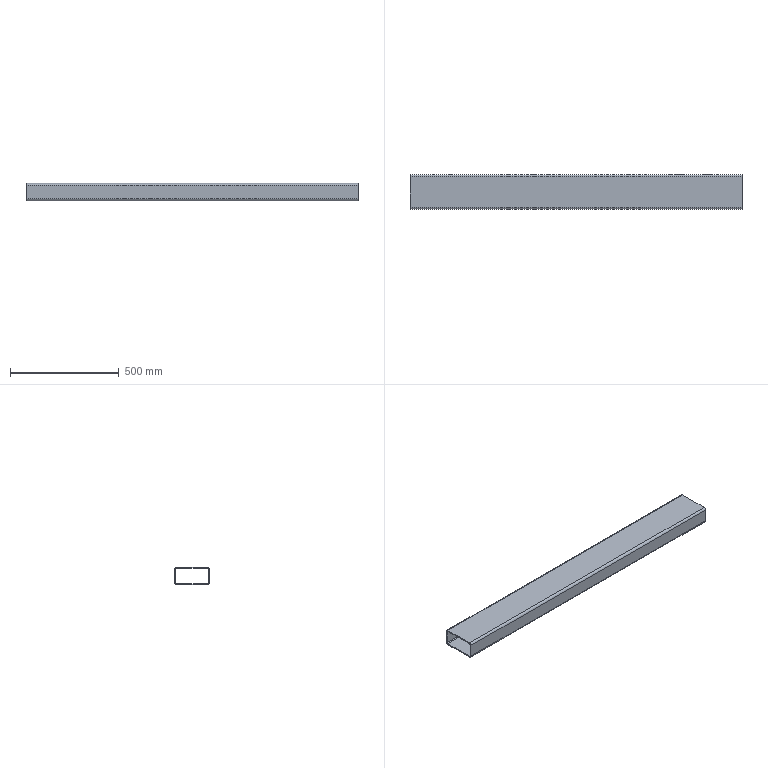Part | SolidWorks | features BaseBody 1 | 1 solid | 42 faces | box 1530 x 160 x 80 mm | volume 3404780 mm3 | cylinder 32 | plane 10 | commonest cylinder face diameters 8.5 x20 10 x4 20 x4 40.497 x4
STEP:
#1=CARTESIAN_POINT('',(324.25,75.,0.));
#2=VERTEX_POINT('',#1);
#3=CARTESIAN_POINT('',(315.75,75.,0.));
#4=VERTEX_POINT('',#3);
#5=CARTESIAN_POINT('',(320.,75.,0.));
#6=DIRECTION('',(0.,-1.,0.));
#7=DIRECTION('',(0.,0.,-1.));
#8=AXIS2_PLACEMENT_3D('',#5,#6,#7);
#9=CIRCLE('',#8,4.25);
#10=EDGE_CURVE('',#2,#4,#9,.T.);
#11=ORIENTED_EDGE('',*,*,#10,.T.);
#12=CARTESIAN_POINT('',(315.75,80.,0.));
#13=VERTEX_POINT('',#12);
#14=CARTESIAN_POINT('',(315.75,90.,0.));
#15=DIRECTION('',(0.,1.,0.));
#16=VECTOR('',#15,1000.);
#17=LINE('',#14,#16);
#18=EDGE_CURVE('',#4,#13,#17,.T.);
#19=ORIENTED_EDGE('',*,*,#18,.T.);
#20=CARTESIAN_POINT('',(324.25,80.,0.));
#21=VERTEX_POINT('',#20);
#22=CARTESIAN_POINT('',(320.,80.,0.));
#23=DIRECTION('',(0.,-1.,0.));
#24=DIRECTION('',(0.,0.,-1.));
#25=AXIS2_PLACEMENT_3D('',#22,#23,#24);
#26=CIRCLE('',#25,4.25);
#27=EDGE_CURVE('',#21,#13,#26,.T.);
#28=ORIENTED_EDGE('',*,*,#27,.F.);
#29=CARTESIAN_POINT('',(324.25,90.,0.));
#30=DIRECTION('',(0.,1.,0.));
#31=VECTOR('',#30,1000.);
#32=LINE('',#29,#31);
#33=EDGE_CURVE('',#2,#21,#32,.T.);
#34=ORIENTED_EDGE('',*,*,#33,.F.);
#35=EDGE_LOOP('',(#11,#19,#28,#34));
#36=FACE_OUTER_BOUND('',#35,.T.);
#37=CARTESIAN_POINT('',(320.,90.,0.));
#38=DIRECTION('',(0.,1.,0.));
#39=DIRECTION('',(1.,0.,0.));
#40=AXIS2_PLACEMENT_3D('',#37,#38,#39);
#41=CYLINDRICAL_SURFACE('',#40,4.25);
#42=ADVANCED_FACE('',(#36),#41,.F.);
#43=CARTESIAN_POINT('',(244.25,75.,0.));
#44=VERTEX_POINT('',#43);
#45=CARTESIAN_POINT('',(235.75,75.,0.));
#46=VERTEX_POINT('',#45);
#47=CARTESIAN_POINT('',(240.,75.,0.));
#48=DIRECTION('',(0.,-1.,0.));
#49=DIRECTION('',(0.,0.,-1.));
#50=AXIS2_PLACEMENT_3D('',#47,#48,#49);
#51=CIRCLE('',#50,4.25);
#52=EDGE_CURVE('',#44,#46,#51,.T.);
#53=ORIENTED_EDGE('',*,*,#52,.T.);
#54=CARTESIAN_POINT('',(235.75,80.,0.));
#55=VERTEX_POINT('',#54);
#56=CARTESIAN_POINT('',(235.75,90.,0.));
#57=DIRECTION('',(0.,1.,0.));
#58=VECTOR('',#57,1000.);
#59=LINE('',#56,#58);
#60=EDGE_CURVE('',#46,#55,#59,.T.);
#61=ORIENTED_EDGE('',*,*,#60,.T.);
#62=CARTESIAN_POINT('',(244.25,80.,0.));
#63=VERTEX_POINT('',#62);
#64=CARTESIAN_POINT('',(240.,80.,0.));
#65=DIRECTION('',(0.,-1.,0.));
#66=DIRECTION('',(0.,0.,-1.));
#67=AXIS2_PLACEMENT_3D('',#64,#65,#66);
#68=CIRCLE('',#67,4.25);
#69=EDGE_CURVE('',#63,#55,#68,.T.);
#70=ORIENTED_EDGE('',*,*,#69,.F.);
#71=CARTESIAN_POINT('',(244.25,90.,0.));
#72=DIRECTION('',(0.,1.,0.));
#73=VECTOR('',#72,1000.);
#74=LINE('',#71,#73);
#75=EDGE_CURVE('',#44,#63,#74,.T.);
#76=ORIENTED_EDGE('',*,*,#75,.F.);
#77=EDGE_LOOP('',(#53,#61,#70,#76));
#78=FACE_OUTER_BOUND('',#77,.T.);
#79=CARTESIAN_POINT('',(240.,90.,0.));
#80=DIRECTION('',(0.,1.,0.));
#81=DIRECTION('',(1.,0.,0.));
#82=AXIS2_PLACEMENT_3D('',#79,#80,#81);
#83=CYLINDRICAL_SURFACE('',#82,4.25);
#84=ADVANCED_FACE('',(#78),#83,.F.);
#85=CARTESIAN_POINT('',(-125.75,75.,0.));
#86=VERTEX_POINT('',#85);
#87=CARTESIAN_POINT('',(-134.25,75.,0.));
#88=VERTEX_POINT('',#87);
#89=CARTESIAN_POINT('',(-130.,75.,0.));
#90=DIRECTION('',(0.,-1.,0.));
#91=DIRECTION('',(0.,0.,-1.));
#92=AXIS2_PLACEMENT_3D('',#89,#90,#91);
#93=CIRCLE('',#92,4.25);
#94=EDGE_CURVE('',#86,#88,#93,.T.);
#95=ORIENTED_EDGE('',*,*,#94,.T.);
#96=CARTESIAN_POINT('',(-134.25,80.,0.));
#97=VERTEX_POINT('',#96);
#98=CARTESIAN_POINT('',(-134.25,90.,0.));
#99=DIRECTION('',(0.,1.,0.));
#100=VECTOR('',#99,1000.);
#101=LINE('',#98,#100);
#102=EDGE_CURVE('',#88,#97,#101,.T.);
#103=ORIENTED_EDGE('',*,*,#102,.T.);
#104=CARTESIAN_POINT('',(-125.75,80.,0.));
#105=VERTEX_POINT('',#104);
#106=CARTESIAN_POINT('',(-130.,80.,0.));
#107=DIRECTION('',(0.,-1.,0.));
#108=DIRECTION('',(0.,0.,-1.));
#109=AXIS2_PLACEMENT_3D('',#106,#107,#108);
#110=CIRCLE('',#109,4.25);
#111=EDGE_CURVE('',#105,#97,#110,.T.);
#112=ORIENTED_EDGE('',*,*,#111,.F.);
#113=CARTESIAN_POINT('',(-125.75,90.,0.));
#114=DIRECTION('',(0.,1.,0.));
#115=VECTOR('',#114,1000.);
#116=LINE('',#113,#115);
#117=EDGE_CURVE('',#86,#105,#116,.T.);
#118=ORIENTED_EDGE('',*,*,#117,.F.);
#119=EDGE_LOOP('',(#95,#103,#112,#118));
#120=FACE_OUTER_BOUND('',#119,.T.);
#121=CARTESIAN_POINT('',(-130.,90.,0.));
#122=DIRECTION('',(0.,1.,0.));
#123=DIRECTION('',(1.,0.,0.));
#124=AXIS2_PLACEMENT_3D('',#121,#122,#123);
#125=CYLINDRICAL_SURFACE('',#124,4.25);
#126=ADVANCED_FACE('',(#120),#125,.F.);
#127=CARTESIAN_POINT('',(-205.75,75.,0.));
#128=VERTEX_POINT('',#127);
#129=CARTESIAN_POINT('',(-214.25,75.,0.));
#130=VERTEX_POINT('',#129);
#131=CARTESIAN_POINT('',(-210.,75.,0.));
#132=DIRECTION('',(0.,-1.,0.));
#133=DIRECTION('',(0.,0.,-1.));
#134=AXIS2_PLACEMENT_3D('',#131,#132,#133);
#135=CIRCLE('',#134,4.25);
#136=EDGE_CURVE('',#128,#130,#135,.T.);
#137=ORIENTED_EDGE('',*,*,#136,.T.);
#138=CARTESIAN_POINT('',(-214.25,80.,0.));
#139=VERTEX_POINT('',#138);
#140=CARTESIAN_POINT('',(-214.25,90.,0.));
#141=DIRECTION('',(0.,1.,0.));
#142=VECTOR('',#141,1000.);
#143=LINE('',#140,#142);
#144=EDGE_CURVE('',#130,#139,#143,.T.);
#145=ORIENTED_EDGE('',*,*,#144,.T.);
#146=CARTESIAN_POINT('',(-205.75,80.,0.));
#147=VERTEX_POINT('',#146);
#148=CARTESIAN_POINT('',(-210.,80.,0.));
#149=DIRECTION('',(0.,-1.,0.));
#150=DIRECTION('',(0.,0.,-1.));
#151=AXIS2_PLACEMENT_3D('',#148,#149,#150);
#152=CIRCLE('',#151,4.25);
#153=EDGE_CURVE('',#147,#139,#152,.T.);
#154=ORIENTED_EDGE('',*,*,#153,.F.);
#155=CARTESIAN_POINT('',(-205.75,90.,0.));
#156=DIRECTION('',(0.,1.,0.));
#157=VECTOR('',#156,1000.);
#158=LINE('',#155,#157);
#159=EDGE_CURVE('',#128,#147,#158,.T.);
#160=ORIENTED_EDGE('',*,*,#159,.F.);
#161=EDGE_LOOP('',(#137,#145,#154,#160));
#162=FACE_OUTER_BOUND('',#161,.T.);
#163=CARTESIAN_POINT('',(-210.,90.,0.));
#164=DIRECTION('',(0.,1.,0.));
#165=DIRECTION('',(1.,0.,0.));
#166=AXIS2_PLACEMENT_3D('',#163,#164,#165);
#167=CYLINDRICAL_SURFACE('',#166,4.25);
#168=ADVANCED_FACE('',(#162),#167,.F.);
#169=CARTESIAN_POINT('',(-575.75,75.,0.));
#170=VERTEX_POINT('',#169);
#171=CARTESIAN_POINT('',(-584.25,75.,0.));
#172=VERTEX_POINT('',#171);
#173=CARTESIAN_POINT('',(-580.,75.,0.));
#174=DIRECTION('',(0.,-1.,0.));
#175=DIRECTION('',(0.,0.,-1.));
#176=AXIS2_PLACEMENT_3D('',#173,#174,#175);
#177=CIRCLE('',#176,4.25);
#178=EDGE_CURVE('',#170,#172,#177,.T.);
#179=ORIENTED_EDGE('',*,*,#178,.T.);
#180=CARTESIAN_POINT('',(-584.25,80.,0.));
#181=VERTEX_POINT('',#180);
#182=CARTESIAN_POINT('',(-584.25,90.,0.));
#183=DIRECTION('',(0.,1.,0.));
#184=VECTOR('',#183,1000.);
#185=LINE('',#182,#184);
#186=EDGE_CURVE('',#172,#181,#185,.T.);
#187=ORIENTED_EDGE('',*,*,#186,.T.);
#188=CARTESIAN_POINT('',(-575.75,80.,0.));
#189=VERTEX_POINT('',#188);
#190=CARTESIAN_POINT('',(-580.,80.,0.));
#191=DIRECTION('',(0.,-1.,0.));
#192=DIRECTION('',(0.,0.,-1.));
#193=AXIS2_PLACEMENT_3D('',#190,#191,#192);
#194=CIRCLE('',#193,4.25);
#195=EDGE_CURVE('',#189,#181,#194,.T.);
#196=ORIENTED_EDGE('',*,*,#195,.F.);
#197=CARTESIAN_POINT('',(-575.75,90.,0.));
#198=DIRECTION('',(0.,1.,0.));
#199=VECTOR('',#198,1000.);
#200=LINE('',#197,#199);
#201=EDGE_CURVE('',#170,#189,#200,.T.);
#202=ORIENTED_EDGE('',*,*,#201,.F.);
#203=EDGE_LOOP('',(#179,#187,#196,#202));
#204=FACE_OUTER_BOUND('',#203,.T.);
#205=CARTESIAN_POINT('',(-580.,90.,0.));
#206=DIRECTION('',(0.,1.,0.));
#207=DIRECTION('',(1.,0.,0.));
#208=AXIS2_PLACEMENT_3D('',#205,#206,#207);
#209=CYLINDRICAL_SURFACE('',#208,4.25);
#210=ADVANCED_FACE('',(#204),#209,.F.);
#211=CARTESIAN_POINT('',(-655.75,75.,0.));
#212=VERTEX_POINT('',#211);
#213=CARTESIAN_POINT('',(-664.25,75.,0.));
#214=VERTEX_POINT('',#213);
#215=CARTESIAN_POINT('',(-660.,75.,0.));
#216=DIRECTION('',(0.,-1.,0.));
#217=DIRECTION('',(0.,0.,-1.));
#218=AXIS2_PLACEMENT_3D('',#215,#216,#217);
#219=CIRCLE('',#218,4.25);
#220=EDGE_CURVE('',#212,#214,#219,.T.);
#221=ORIENTED_EDGE('',*,*,#220,.T.);
#222=CARTESIAN_POINT('',(-664.25,80.,0.));
#223=VERTEX_POINT('',#222);
#224=CARTESIAN_POINT('',(-664.25,90.,0.));
#225=DIRECTION('',(0.,1.,0.));
#226=VECTOR('',#225,1000.);
#227=LINE('',#224,#226);
#228=EDGE_CURVE('',#214,#223,#227,.T.);
#229=ORIENTED_EDGE('',*,*,#228,.T.);
#230=CARTESIAN_POINT('',(-655.75,80.,0.));
#231=VERTEX_POINT('',#230);
#232=CARTESIAN_POINT('',(-660.,80.,0.));
#233=DIRECTION('',(0.,-1.,0.));
#234=DIRECTION('',(0.,0.,-1.));
#235=AXIS2_PLACEMENT_3D('',#232,#233,#234);
#236=CIRCLE('',#235,4.25);
#237=EDGE_CURVE('',#231,#223,#236,.T.);
#238=ORIENTED_EDGE('',*,*,#237,.F.);
#239=CARTESIAN_POINT('',(-655.75,90.,0.));
#240=DIRECTION('',(0.,1.,0.));
#241=VECTOR('',#240,1000.);
#242=LINE('',#239,#241);
#243=EDGE_CURVE('',#212,#231,#242,.T.);
#244=ORIENTED_EDGE('',*,*,#243,.F.);
#245=EDGE_LOOP('',(#221,#229,#238,#244));
#246=FACE_OUTER_BOUND('',#245,.T.);
#247=CARTESIAN_POINT('',(-660.,90.,0.));
#248=DIRECTION('',(0.,1.,0.));
#249=DIRECTION('',(1.,0.,0.));
#250=AXIS2_PLACEMENT_3D('',#247,#248,#249);
#251=CYLINDRICAL_SURFACE('',#250,4.25);
#252=ADVANCED_FACE('',(#246),#251,.F.);
#253=CARTESIAN_POINT('',(627.748,75.,0.));
#254=VERTEX_POINT('',#253);
#255=CARTESIAN_POINT('',(587.252,75.,0.));
#256=VERTEX_POINT('',#255);
#257=CARTESIAN_POINT('',(607.5,75.,0.));
#258=DIRECTION('',(0.,-1.,0.));
#259=DIRECTION('',(0.,0.,-1.));
#260=AXIS2_PLACEMENT_3D('',#257,#258,#259);
#261=CIRCLE('',#260,20.248);
#262=EDGE_CURVE('',#254,#256,#261,.T.);
#263=ORIENTED_EDGE('',*,*,#262,.T.);
#264=CARTESIAN_POINT('',(587.252,80.,0.));
#265=VERTEX_POINT('',#264);
#266=CARTESIAN_POINT('',(587.252,70.,0.));
#267=DIRECTION('',(0.,1.,0.));
#268=VECTOR('',#267,1000.);
#269=LINE('',#266,#268);
#270=EDGE_CURVE('',#256,#265,#269,.T.);
#271=ORIENTED_EDGE('',*,*,#270,.T.);
#272=CARTESIAN_POINT('',(627.748,80.,0.));
#273=VERTEX_POINT('',#272);
#274=CARTESIAN_POINT('',(607.5,80.,0.));
#275=DIRECTION('',(0.,-1.,0.));
#276=DIRECTION('',(0.,0.,-1.));
#277=AXIS2_PLACEMENT_3D('',#274,#275,#276);
#278=CIRCLE('',#277,20.248);
#279=EDGE_CURVE('',#273,#265,#278,.T.);
#280=ORIENTED_EDGE('',*,*,#279,.F.);
#281=CARTESIAN_POINT('',(627.748,70.,0.));
#282=DIRECTION('',(0.,1.,0.));
#283=VECTOR('',#282,1000.);
#284=LINE('',#281,#283);
#285=EDGE_CURVE('',#254,#273,#284,.T.);
#286=ORIENTED_EDGE('',*,*,#285,.F.);
#287=EDGE_LOOP('',(#263,#271,#280,#286));
#288=FACE_OUTER_BOUND('',#287,.T.);
#289=CARTESIAN_POINT('',(607.5,70.,0.));
#290=DIRECTION('',(0.,1.,0.));
#291=DIRECTION('',(1.,0.,0.));
#292=AXIS2_PLACEMENT_3D('',#289,#290,#291);
#293=CYLINDRICAL_SURFACE('',#292,20.248);
#294=ADVANCED_FACE('',(#288),#293,.F.);
#295=CARTESIAN_POINT('',(492.748,75.,0.));
#296=VERTEX_POINT('',#295);
#297=CARTESIAN_POINT('',(452.252,75.,0.));
#298=VERTEX_POINT('',#297);
#299=CARTESIAN_POINT('',(472.5,75.,0.));
#300=DIRECTION('',(0.,-1.,0.));
#301=DIRECTION('',(0.,0.,-1.));
#302=AXIS2_PLACEMENT_3D('',#299,#300,#301);
#303=CIRCLE('',#302,20.248);
#304=EDGE_CURVE('',#296,#298,#303,.T.);
#305=ORIENTED_EDGE('',*,*,#304,.T.);
#306=CARTESIAN_POINT('',(452.252,80.,0.));
#307=VERTEX_POINT('',#306);
#308=CARTESIAN_POINT('',(452.252,70.,0.));
#309=DIRECTION('',(0.,1.,0.));
#310=VECTOR('',#309,1000.);
#311=LINE('',#308,#310);
#312=EDGE_CURVE('',#298,#307,#311,.T.);
#313=ORIENTED_EDGE('',*,*,#312,.T.);
#314=CARTESIAN_POINT('',(492.748,80.,0.));
#315=VERTEX_POINT('',#314);
#316=CARTESIAN_POINT('',(472.5,80.,0.));
#317=DIRECTION('',(0.,-1.,0.));
#318=DIRECTION('',(0.,0.,-1.));
#319=AXIS2_PLACEMENT_3D('',#316,#317,#318);
#320=CIRCLE('',#319,20.248);
#321=EDGE_CURVE('',#315,#307,#320,.T.);
#322=ORIENTED_EDGE('',*,*,#321,.F.);
#323=CARTESIAN_POINT('',(492.748,70.,0.));
#324=DIRECTION('',(0.,1.,0.));
#325=VECTOR('',#324,1000.);
#326=LINE('',#323,#325);
#327=EDGE_CURVE('',#296,#315,#326,.T.);
#328=ORIENTED_EDGE('',*,*,#327,.F.);
#329=EDGE_LOOP('',(#305,#313,#322,#328));
#330=FACE_OUTER_BOUND('',#329,.T.);
#331=CARTESIAN_POINT('',(472.5,70.,0.));
#332=DIRECTION('',(0.,1.,0.));
#333=DIRECTION('',(1.,0.,0.));
#334=AXIS2_PLACEMENT_3D('',#331,#332,#333);
#335=CYLINDRICAL_SURFACE('',#334,20.248);
#336=ADVANCED_FACE('',(#330),#335,.F.);
#337=CARTESIAN_POINT('',(436.75,75.,-15.));
#338=VERTEX_POINT('',#337);
#339=CARTESIAN_POINT('',(428.25,75.,-15.));
#340=VERTEX_POINT('',#339);
#341=CARTESIAN_POINT('',(432.5,75.,-15.));
#342=DIRECTION('',(0.,-1.,0.));
#343=DIRECTION('',(0.,0.,-1.));
#344=AXIS2_PLACEMENT_3D('',#341,#342,#343);
#345=CIRCLE('',#344,4.25);
#346=EDGE_CURVE('',#338,#340,#345,.T.);
#347=ORIENTED_EDGE('',*,*,#346,.T.);
#348=CARTESIAN_POINT('',(428.25,80.,-15.));
#349=VERTEX_POINT('',#348);
#350=CARTESIAN_POINT('',(428.25,90.,-15.));
#351=DIRECTION('',(0.,1.,0.));
#352=VECTOR('',#351,1000.);
#353=LINE('',#350,#352);
#354=EDGE_CURVE('',#340,#349,#353,.T.);
#355=ORIENTED_EDGE('',*,*,#354,.T.);
#356=CARTESIAN_POINT('',(436.75,80.,-15.));
#357=VERTEX_POINT('',#356);
#358=CARTESIAN_POINT('',(432.5,80.,-15.));
#359=DIRECTION('',(0.,-1.,0.));
#360=DIRECTION('',(0.,0.,-1.));
#361=AXIS2_PLACEMENT_3D('',#358,#359,#360);
#362=CIRCLE('',#361,4.25);
#363=EDGE_CURVE('',#357,#349,#362,.T.);
#364=ORIENTED_EDGE('',*,*,#363,.F.);
#365=CARTESIAN_POINT('',(436.75,90.,-15.));
#366=DIRECTION('',(0.,1.,0.));
#367=VECTOR('',#366,1000.);
#368=LINE('',#365,#367);
#369=EDGE_CURVE('',#338,#357,#368,.T.);
#370=ORIENTED_EDGE('',*,*,#369,.F.);
#371=EDGE_LOOP('',(#347,#355,#364,#370));
#372=FACE_OUTER_BOUND('',#371,.T.);
#373=CARTESIAN_POINT('',(432.5,90.,-15.));
#374=DIRECTION('',(0.,1.,0.));
#375=DIRECTION('',(1.,0.,0.));
#376=AXIS2_PLACEMENT_3D('',#373,#374,#375);
#377=CYLINDRICAL_SURFACE('',#376,4.25);
#378=ADVANCED_FACE('',(#372),#377,.F.);
#379=CARTESIAN_POINT('',(436.75,75.,15.));
#380=VERTEX_POINT('',#379);
#381=CARTESIAN_POINT('',(428.25,75.,15.));
#382=VERTEX_POINT('',#381);
#383=CARTESIAN_POINT('',(432.5,75.,15.));
#384=DIRECTION('',(0.,-1.,0.));
#385=DIRECTION('',(0.,0.,-1.));
#386=AXIS2_PLACEMENT_3D('',#383,#384,#385);
#387=CIRCLE('',#386,4.25);
#388=EDGE_CURVE('',#380,#382,#387,.T.);
#389=ORIENTED_EDGE('',*,*,#388,.T.);
#390=CARTESIAN_POINT('',(428.25,80.,15.));
#391=VERTEX_POINT('',#390);
#392=CARTESIAN_POINT('',(428.25,90.,15.));
#393=DIRECTION('',(0.,1.,0.));
#394=VECTOR('',#393,1000.);
#395=LINE('',#392,#394);
#396=EDGE_CURVE('',#382,#391,#395,.T.);
#397=ORIENTED_EDGE('',*,*,#396,.T.);
#398=CARTESIAN_POINT('',(436.75,80.,15.));
#399=VERTEX_POINT('',#398);
#400=CARTESIAN_POINT('',(432.5,80.,15.));
#401=DIRECTION('',(0.,-1.,0.));
#402=DIRECTION('',(0.,0.,-1.));
#403=AXIS2_PLACEMENT_3D('',#400,#401,#402);
#404=CIRCLE('',#403,4.25);
#405=EDGE_CURVE('',#399,#391,#404,.T.);
#406=ORIENTED_EDGE('',*,*,#405,.F.);
#407=CARTESIAN_POINT('',(436.75,90.,15.));
#408=DIRECTION('',(0.,1.,0.));
#409=VECTOR('',#408,1000.);
#410=LINE('',#407,#409);
#411=EDGE_CURVE('',#380,#399,#410,.T.);
#412=ORIENTED_EDGE('',*,*,#411,.F.);
#413=EDGE_LOOP('',(#389,#397,#406,#412));
#414=FACE_OUTER_BOUND('',#413,.T.);
#415=CARTESIAN_POINT('',(432.5,90.,15.));
#416=DIRECTION('',(0.,1.,0.));
#417=DIRECTION('',(1.,0.,0.));
#418=AXIS2_PLACEMENT_3D('',#415,#416,#417);
#419=CYLINDRICAL_SURFACE('',#418,4.25);
#420=ADVANCED_FACE('',(#414),#419,.F.);
#421=CARTESIAN_POINT('',(651.75,75.,15.));
#422=VERTEX_POINT('',#421);
#423=CARTESIAN_POINT('',(643.25,75.,15.));
#424=VERTEX_POINT('',#423);
#425=CARTESIAN_POINT('',(647.5,75.,15.));
#426=DIRECTION('',(0.,-1.,0.));
#427=DIRECTION('',(0.,0.,-1.));
#428=AXIS2_PLACEMENT_3D('',#425,#426,#427);
#429=CIRCLE('',#428,4.25);
#430=EDGE_CURVE('',#422,#424,#429,.T.);
#431=ORIENTED_EDGE('',*,*,#430,.T.);
#432=CARTESIAN_POINT('',(643.25,80.,15.));
#433=VERTEX_POINT('',#432);
#434=CARTESIAN_POINT('',(643.25,90.,15.));
#435=DIRECTION('',(0.,1.,0.));
#436=VECTOR('',#435,1000.);
#437=LINE('',#434,#436);
#438=EDGE_CURVE('',#424,#433,#437,.T.);
#439=ORIENTED_EDGE('',*,*,#438,.T.);
#440=CARTESIAN_POINT('',(651.75,80.,15.));
#441=VERTEX_POINT('',#440);
#442=CARTESIAN_POINT('',(647.5,80.,15.));
#443=DIRECTION('',(0.,-1.,0.));
#444=DIRECTION('',(0.,0.,-1.));
#445=AXIS2_PLACEMENT_3D('',#442,#443,#444);
#446=CIRCLE('',#445,4.25);
#447=EDGE_CURVE('',#441,#433,#446,.T.);
#448=ORIENTED_EDGE('',*,*,#447,.F.);
#449=CARTESIAN_POINT('',(651.75,90.,15.));
#450=DIRECTION('',(0.,1.,0.));
#451=VECTOR('',#450,1000.);
#452=LINE('',#449,#451);
#453=EDGE_CURVE('',#422,#441,#452,.T.);
#454=ORIENTED_EDGE('',*,*,#453,.F.);
#455=EDGE_LOOP('',(#431,#439,#448,#454));
#456=FACE_OUTER_BOUND('',#455,.T.);
#457=CARTESIAN_POINT('',(647.5,90.,15.));
#458=DIRECTION('',(0.,1.,0.));
#459=DIRECTION('',(1.,0.,0.));
#460=AXIS2_PLACEMENT_3D('',#457,#458,#459);
#461=CYLINDRICAL_SURFACE('',#460,4.25);
#462=ADVANCED_FACE('',(#456),#461,.F.);
#463=CARTESIAN_POINT('',(651.75,75.,-15.));
#464=VERTEX_POINT('',#463);
#465=CARTESIAN_POINT('',(643.25,75.,-15.));
#466=VERTEX_POINT('',#465);
#467=CARTESIAN_POINT('',(647.5,75.,-15.));
#468=DIRECTION('',(0.,-1.,0.));
#469=DIRECTION('',(0.,0.,-1.));
#470=AXIS2_PLACEMENT_3D('',#467,#468,#469);
#471=CIRCLE('',#470,4.25);
#472=EDGE_CURVE('',#464,#466,#471,.T.);
#473=ORIENTED_EDGE('',*,*,#472,.T.);
#474=CARTESIAN_POINT('',(643.25,80.,-15.));
#475=VERTEX_POINT('',#474);
#476=CARTESIAN_POINT('',(643.25,90.,-15.));
#477=DIRECTION('',(0.,1.,0.));
#478=VECTOR('',#477,1000.);
#479=LINE('',#476,#478);
#480=EDGE_CURVE('',#466,#475,#479,.T.);
#481=ORIENTED_EDGE('',*,*,#480,.T.);
#482=CARTESIAN_POINT('',(651.75,80.,-15.));
#483=VERTEX_POINT('',#482);
#484=CARTESIAN_POINT('',(647.5,80.,-15.));
#485=DIRECTION('',(0.,-1.,0.));
#486=DIRECTION('',(0.,0.,-1.));
#487=AXIS2_PLACEMENT_3D('',#484,#485,#486);
#488=CIRCLE('',#487,4.25);
#489=EDGE_CURVE('',#483,#475,#488,.T.);
#490=ORIENTED_EDGE('',*,*,#489,.F.);
#491=CARTESIAN_POINT('',(651.75,90.,-15.));
#492=DIRECTION('',(0.,1.,0.));
#493=VECTOR('',#492,1000.);
#494=LINE('',#491,#493);
#495=EDGE_CURVE('',#464,#483,#494,.T.);
#496=ORIENTED_EDGE('',*,*,#495,.F.);
#497=EDGE_LOOP('',(#473,#481,#490,#496));
#498=FACE_OUTER_BOUND('',#497,.T.);
#499=CARTESIAN_POINT('',(647.5,90.,-15.));
#500=DIRECTION('',(0.,1.,0.));
#501=DIRECTION('',(1.,0.,0.));
#502=AXIS2_PLACEMENT_3D('',#499,#500,#501);
#503=CYLINDRICAL_SURFACE('',#502,4.25);
#504=ADVANCED_FACE('',(#498),#503,.F.);
#505=CARTESIAN_POINT('',(762.5,70.,-40.));
#506=VERTEX_POINT('',#505);
#507=CARTESIAN_POINT('',(762.5,80.,-30.));
#508=VERTEX_POINT('',#507);
#509=CARTESIAN_POINT('',(762.5,70.,-30.));
#510=DIRECTION('',(1.,0.,0.));
#511=DIRECTION('',(0.,1.,0.));
#512=AXIS2_PLACEMENT_3D('',#509,#510,#511);
#513=CIRCLE('',#512,10.);
#514=EDGE_CURVE('',#506,#508,#513,.T.);
#515=ORIENTED_EDGE('',*,*,#514,.F.);
#516=CARTESIAN_POINT('',(-767.5,70.,-40.));
#517=VERTEX_POINT('',#516);
#518=CARTESIAN_POINT('',(767.5,70.,-40.));
#519=DIRECTION('',(-1.,0.,0.));
#520=VECTOR('',#519,1000.);
#521=LINE('',#518,#520);
#522=EDGE_CURVE('',#506,#517,#521,.T.);
#523=ORIENTED_EDGE('',*,*,#522,.T.);
#524=CARTESIAN_POINT('',(-767.5,80.,-30.));
#525=VERTEX_POINT('',#524);
#526=CARTESIAN_POINT('',(-767.5,70.,-30.));
#527=DIRECTION('',(1.,0.,0.));
#528=DIRECTION('',(0.,0.,-1.));
#529=AXIS2_PLACEMENT_3D('',#526,#527,#528);
#530=CIRCLE('',#529,10.);
#531=EDGE_CURVE('',#517,#525,#530,.T.);
#532=ORIENTED_EDGE('',*,*,#531,.T.);
#533=CARTESIAN_POINT('',(767.5,80.,-30.));
#534=DIRECTION('',(-1.,0.,0.));
#535=VECTOR('',#534,1000.);
#536=LINE('',#533,#535);
#537=EDGE_CURVE('',#508,#525,#536,.T.);
#538=ORIENTED_EDGE('',*,*,#537,.F.);
#539=EDGE_LOOP('',(#515,#523,#532,#538));
#540=FACE_OUTER_BOUND('',#539,.T.);
#541=CARTESIAN_POINT('',(767.5,70.,-30.));
#542=DIRECTION('',(-1.,0.,0.));
#543=DIRECTION('',(0.,0.,1.));
#544=AXIS2_PLACEMENT_3D('',#541,#542,#543);
#545=CYLINDRICAL_SURFACE('',#544,10.);
#546=ADVANCED_FACE('',(#540),#545,.T.);
#547=ORIENTED_EDGE('',*,*,#27,.T.);
#548=CARTESIAN_POINT('',(320.,80.,0.));
#549=DIRECTION('',(0.,-1.,0.));
#550=DIRECTION('',(0.,0.,-1.));
#551=AXIS2_PLACEMENT_3D('',#548,#549,#550);
#552=CIRCLE('',#551,4.25);
#553=EDGE_CURVE('',#13,#21,#552,.T.);
#554=ORIENTED_EDGE('',*,*,#553,.T.);
#555=EDGE_LOOP('',(#547,#554));
#556=FACE_BOUND('',#555,.T.);
#557=ORIENTED_EDGE('',*,*,#69,.T.);
#558=CARTESIAN_POINT('',(240.,80.,0.));
#559=DIRECTION('',(0.,-1.,0.));
#560=DIRECTION('',(0.,0.,-1.));
#561=AXIS2_PLACEMENT_3D('',#558,#559,#560);
#562=CIRCLE('',#561,4.25);
#563=EDGE_CURVE('',#55,#63,#562,.T.);
#564=ORIENTED_EDGE('',*,*,#563,.T.);
#565=EDGE_LOOP('',(#557,#564));
#566=FACE_BOUND('',#565,.T.);
#567=ORIENTED_EDGE('',*,*,#111,.T.);
#568=CARTESIAN_POINT('',(-130.,80.,0.));
#569=DIRECTION('',(0.,-1.,0.));
#570=DIRECTION('',(0.,0.,-1.));
#571=AXIS2_PLACEMENT_3D('',#568,#569,#570);
#572=CIRCLE('',#571,4.25);
#573=EDGE_CURVE('',#97,#105,#572,.T.);
#574=ORIENTED_EDGE('',*,*,#573,.T.);
#575=EDGE_LOOP('',(#567,#574));
#576=FACE_BOUND('',#575,.T.);
#577=ORIENTED_EDGE('',*,*,#153,.T.);
#578=CARTESIAN_POINT('',(-210.,80.,0.));
#579=DIRECTION('',(0.,-1.,0.));
#580=DIRECTION('',(0.,0.,-1.));
#581=AXIS2_PLACEMENT_3D('',#578,#579,#580);
#582=CIRCLE('',#581,4.25);
#583=EDGE_CURVE('',#139,#147,#582,.T.);
#584=ORIENTED_EDGE('',*,*,#583,.T.);
#585=EDGE_LOOP('',(#577,#584));
#586=FACE_BOUND('',#585,.T.);
#587=ORIENTED_EDGE('',*,*,#195,.T.);
#588=CARTESIAN_POINT('',(-580.,80.,0.));
#589=DIRECTION('',(0.,-1.,0.));
#590=DIRECTION('',(0.,0.,-1.));
#591=AXIS2_PLACEMENT_3D('',#588,#589,#590);
#592=CIRCLE('',#591,4.25);
#593=EDGE_CURVE('',#181,#189,#592,.T.);
#594=ORIENTED_EDGE('',*,*,#593,.T.);
#595=EDGE_LOOP('',(#587,#594));
#596=FACE_BOUND('',#595,.T.);
#597=ORIENTED_EDGE('',*,*,#237,.T.);
#598=CARTESIAN_POINT('',(-660.,80.,0.));
#599=DIRECTION('',(0.,-1.,0.));
#600=DIRECTION('',(0.,0.,-1.));
#601=AXIS2_PLACEMENT_3D('',#598,#599,#600);
#602=CIRCLE('',#601,4.25);
#603=EDGE_CURVE('',#223,#231,#602,.T.);
#604=ORIENTED_EDGE('',*,*,#603,.T.);
#605=EDGE_LOOP('',(#597,#604));
#606=FACE_BOUND('',#605,.T.);
#607=ORIENTED_EDGE('',*,*,#279,.T.);
#608=CARTESIAN_POINT('',(607.5,80.,0.));
#609=DIRECTION('',(0.,-1.,0.));
#610=DIRECTION('',(0.,0.,-1.));
#611=AXIS2_PLACEMENT_3D('',#608,#609,#610);
#612=CIRCLE('',#611,20.248);
#613=EDGE_CURVE('',#265,#273,#612,.T.);
#614=ORIENTED_EDGE('',*,*,#613,.T.);
#615=EDGE_LOOP('',(#607,#614));
#616=FACE_BOUND('',#615,.T.);
#617=ORIENTED_EDGE('',*,*,#321,.T.);
#618=CARTESIAN_POINT('',(472.5,80.,0.));
#619=DIRECTION('',(0.,-1.,0.));
#620=DIRECTION('',(0.,0.,-1.));
#621=AXIS2_PLACEMENT_3D('',#618,#619,#620);
#622=CIRCLE('',#621,20.248);
#623=EDGE_CURVE('',#307,#315,#622,.T.);
#624=ORIENTED_EDGE('',*,*,#623,.T.);
#625=EDGE_LOOP('',(#617,#624));
#626=FACE_BOUND('',#625,.T.);
#627=ORIENTED_EDGE('',*,*,#363,.T.);
#628=CARTESIAN_POINT('',(432.5,80.,-15.));
#629=DIRECTION('',(0.,-1.,0.));
#630=DIRECTION('',(0.,0.,-1.));
#631=AXIS2_PLACEMENT_3D('',#628,#629,#630);
#632=CIRCLE('',#631,4.25);
#633=EDGE_CURVE('',#349,#357,#632,.T.);
#634=ORIENTED_EDGE('',*,*,#633,.T.);
#635=EDGE_LOOP('',(#627,#634));
#636=FACE_BOUND('',#635,.T.);
#637=ORIENTED_EDGE('',*,*,#405,.T.);
#638=CARTESIAN_POINT('',(432.5,80.,15.));
#639=DIRECTION('',(0.,-1.,0.));
#640=DIRECTION('',(0.,0.,-1.));
#641=AXIS2_PLACEMENT_3D('',#638,#639,#640);
#642=CIRCLE('',#641,4.25);
#643=EDGE_CURVE('',#391,#399,#642,.T.);
#644=ORIENTED_EDGE('',*,*,#643,.T.);
#645=EDGE_LOOP('',(#637,#644));
#646=FACE_BOUND('',#645,.T.);
#647=ORIENTED_EDGE('',*,*,#447,.T.);
#648=CARTESIAN_POINT('',(647.5,80.,15.));
#649=DIRECTION('',(0.,-1.,0.));
#650=DIRECTION('',(0.,0.,-1.));
#651=AXIS2_PLACEMENT_3D('',#648,#649,#650);
#652=CIRCLE('',#651,4.25);
#653=EDGE_CURVE('',#433,#441,#652,.T.);
#654=ORIENTED_EDGE('',*,*,#653,.T.);
#655=EDGE_LOOP('',(#647,#654));
#656=FACE_BOUND('',#655,.T.);
#657=ORIENTED_EDGE('',*,*,#489,.T.);
#658=CARTESIAN_POINT('',(647.5,80.,-15.));
#659=DIRECTION('',(0.,-1.,0.));
#660=DIRECTION('',(0.,0.,-1.));
#661=AXIS2_PLACEMENT_3D('',#658,#659,#660);
#662=CIRCLE('',#661,4.25);
#663=EDGE_CURVE('',#475,#483,#662,.T.);
#664=ORIENTED_EDGE('',*,*,#663,.T.);
#665=EDGE_LOOP('',(#657,#664));
#666=FACE_BOUND('',#665,.T.);
#667=CARTESIAN_POINT('',(762.5,80.,30.));
#668=VERTEX_POINT('',#667);
#669=CARTESIAN_POINT('',(762.5,80.,-30.));
#670=DIRECTION('',(0.,0.,1.));
#671=VECTOR('',#670,1000.);
#672=LINE('',#669,#671);
#673=EDGE_CURVE('',#508,#668,#672,.T.);
#674=ORIENTED_EDGE('',*,*,#673,.F.);
#675=ORIENTED_EDGE('',*,*,#537,.T.);
#676=CARTESIAN_POINT('',(-767.5,80.,30.));
#677=VERTEX_POINT('',#676);
#678=CARTESIAN_POINT('',(-767.5,80.,-30.));
#679=DIRECTION('',(0.,0.,1.));
#680=VECTOR('',#679,1000.);
#681=LINE('',#678,#680);
#682=EDGE_CURVE('',#525,#677,#681,.T.);
#683=ORIENTED_EDGE('',*,*,#682,.T.);
#684=CARTESIAN_POINT('',(767.5,80.,30.));
#685=DIRECTION('',(-1.,0.,0.));
#686=VECTOR('',#685,1000.);
#687=LINE('',#684,#686);
#688=EDGE_CURVE('',#668,#677,#687,.T.);
#689=ORIENTED_EDGE('',*,*,#688,.F.);
#690=EDGE_LOOP('',(#674,#675,#683,#689));
#691=FACE_OUTER_BOUND('',#690,.T.);
#692=CARTESIAN_POINT('',(767.5,80.,-30.));
#693=DIRECTION('',(0.,-1.,0.));
#694=DIRECTION('',(0.,0.,-1.));
#695=AXIS2_PLACEMENT_3D('',#692,#693,#694);
#696=PLANE('',#695);
#697=ADVANCED_FACE('',(#556,#566,#576,#586,#596,#606,#616,#626,#636,#646,#656,#666,#691),#696,.F.);
#698=CARTESIAN_POINT('',(762.5,70.,40.));
#699=VERTEX_POINT('',#698);
#700=CARTESIAN_POINT('',(762.5,70.,30.));
#701=DIRECTION('',(1.,0.,0.));
#702=DIRECTION('',(0.,1.,0.));
#703=AXIS2_PLACEMENT_3D('',#700,#701,#702);
#704=CIRCLE('',#703,10.);
#705=EDGE_CURVE('',#668,#699,#704,.T.);
#706=ORIENTED_EDGE('',*,*,#705,.F.);
#707=ORIENTED_EDGE('',*,*,#688,.T.);
#708=CARTESIAN_POINT('',(-767.5,70.,40.));
#709=VERTEX_POINT('',#708);
#710=CARTESIAN_POINT('',(-767.5,70.,30.));
#711=DIRECTION('',(1.,0.,0.));
#712=DIRECTION('',(0.,0.,-1.));
#713=AXIS2_PLACEMENT_3D('',#710,#711,#712);
#714=CIRCLE('',#713,10.);
#715=EDGE_CURVE('',#677,#709,#714,.T.);
#716=ORIENTED_EDGE('',*,*,#715,.T.);
#717=CARTESIAN_POINT('',(767.5,70.,40.));
#718=DIRECTION('',(-1.,0.,0.));
#719=VECTOR('',#718,1000.);
#720=LINE('',#717,#719);
#721=EDGE_CURVE('',#699,#709,#720,.T.);
#722=ORIENTED_EDGE('',*,*,#721,.F.);
#723=EDGE_LOOP('',(#706,#707,#716,#722));
#724=FACE_OUTER_BOUND('',#723,.T.);
#725=CARTESIAN_POINT('',(767.5,70.,30.));
#726=DIRECTION('',(-1.,0.,0.));
#727=DIRECTION('',(0.,0.,1.));
#728=AXIS2_PLACEMENT_3D('',#725,#726,#727);
#729=CYLINDRICAL_SURFACE('',#728,10.);
#730=ADVANCED_FACE('',(#724),#729,.T.);
#731=CARTESIAN_POINT('',(762.5,-70.,40.));
#732=VERTEX_POINT('',#731);
#733=CARTESIAN_POINT('',(762.5,-70.,40.));
#734=DIRECTION('',(0.,-1.,0.));
#735=VECTOR('',#734,1000.);
#736=LINE('',#733,#735);
#737=EDGE_CURVE('',#699,#732,#736,.T.);
#738=ORIENTED_EDGE('',*,*,#737,.F.);
#739=ORIENTED_EDGE('',*,*,#721,.T.);
#740=CARTESIAN_POINT('',(-767.5,-70.,40.));
#741=VERTEX_POINT('',#740);
#742=CARTESIAN_POINT('',(-767.5,-70.,40.));
#743=DIRECTION('',(0.,-1.,0.));
#744=VECTOR('',#743,1000.);
#745=LINE('',#742,#744);
#746=EDGE_CURVE('',#709,#741,#745,.T.);
#747=ORIENTED_EDGE('',*,*,#746,.T.);
#748=CARTESIAN_POINT('',(767.5,-70.,40.));
#749=DIRECTION('',(-1.,0.,0.));
#750=VECTOR('',#749,1000.);
#751=LINE('',#748,#750);
#752=EDGE_CURVE('',#732,#741,#751,.T.);
#753=ORIENTED_EDGE('',*,*,#752,.F.);
#754=EDGE_LOOP('',(#738,#739,#747,#753));
#755=FACE_OUTER_BOUND('',#754,.T.);
#756=CARTESIAN_POINT('',(767.5,-70.,40.));
#757=DIRECTION('',(0.,0.,-1.));
#758=DIRECTION('',(-1.,0.,0.));
#759=AXIS2_PLACEMENT_3D('',#756,#757,#758);
#760=PLANE('',#759);
#761=ADVANCED_FACE('',(#755),#760,.F.);
#762=CARTESIAN_POINT('',(762.5,-80.,30.));
#763=VERTEX_POINT('',#762);
#764=CARTESIAN_POINT('',(762.5,-70.,30.));
#765=DIRECTION('',(1.,0.,0.));
#766=DIRECTION('',(0.,1.,0.));
#767=AXIS2_PLACEMENT_3D('',#764,#765,#766);
#768=CIRCLE('',#767,10.);
#769=EDGE_CURVE('',#732,#763,#768,.T.);
#770=ORIENTED_EDGE('',*,*,#769,.F.);
#771=ORIENTED_EDGE('',*,*,#752,.T.);
#772=CARTESIAN_POINT('',(-767.5,-80.,30.));
#773=VERTEX_POINT('',#772);
#774=CARTESIAN_POINT('',(-767.5,-70.,30.));
#775=DIRECTION('',(1.,0.,0.));
#776=DIRECTION('',(0.,0.,-1.));
#777=AXIS2_PLACEMENT_3D('',#774,#775,#776);
#778=CIRCLE('',#777,10.);
#779=EDGE_CURVE('',#741,#773,#778,.T.);
#780=ORIENTED_EDGE('',*,*,#779,.T.);
#781=CARTESIAN_POINT('',(767.5,-80.,30.));
#782=DIRECTION('',(-1.,0.,0.));
#783=VECTOR('',#782,1000.);
#784=LINE('',#781,#783);
#785=EDGE_CURVE('',#763,#773,#784,.T.);
#786=ORIENTED_EDGE('',*,*,#785,.F.);
#787=EDGE_LOOP('',(#770,#771,#780,#786));
#788=FACE_OUTER_BOUND('',#787,.T.);
#789=CARTESIAN_POINT('',(767.5,-70.,30.));
#790=DIRECTION('',(-1.,0.,0.));
#791=DIRECTION('',(0.,0.,1.));
#792=AXIS2_PLACEMENT_3D('',#789,#790,#791);
#793=CYLINDRICAL_SURFACE('',#792,10.);
#794=ADVANCED_FACE('',(#788),#793,.T.);
#795=CARTESIAN_POINT('',(762.5,-80.,-30.));
#796=VERTEX_POINT('',#795);
#797=CARTESIAN_POINT('',(762.5,-80.,1390.));
#798=DIRECTION('',(0.,0.,-1.));
#799=VECTOR('',#798,1000.);
#800=LINE('',#797,#799);
#801=EDGE_CURVE('',#763,#796,#800,.T.);
#802=ORIENTED_EDGE('',*,*,#801,.F.);
#803=ORIENTED_EDGE('',*,*,#785,.T.);
#804=CARTESIAN_POINT('',(-767.5,-80.,-30.));
#805=VERTEX_POINT('',#804);
#806=CARTESIAN_POINT('',(-767.5,-80.,30.));
#807=DIRECTION('',(0.,0.,-1.));
#808=VECTOR('',#807,1000.);
#809=LINE('',#806,#808);
#810=EDGE_CURVE('',#773,#805,#809,.T.);
#811=ORIENTED_EDGE('',*,*,#810,.T.);
#812=CARTESIAN_POINT('',(767.5,-80.,-30.));
#813=DIRECTION('',(-1.,0.,0.));
#814=VECTOR('',#813,1000.);
#815=LINE('',#812,#814);
#816=EDGE_CURVE('',#796,#805,#815,.T.);
#817=ORIENTED_EDGE('',*,*,#816,.F.);
#818=EDGE_LOOP('',(#802,#803,#811,#817));
#819=FACE_OUTER_BOUND('',#818,.T.);
#820=CARTESIAN_POINT('',(767.5,-80.,30.));
#821=DIRECTION('',(0.,1.,0.));
#822=DIRECTION('',(0.,0.,1.));
#823=AXIS2_PLACEMENT_3D('',#820,#821,#822);
#824=PLANE('',#823);
#825=ADVANCED_FACE('',(#819),#824,.F.);
#826=CARTESIAN_POINT('',(762.5,-70.,-40.));
#827=VERTEX_POINT('',#826);
#828=CARTESIAN_POINT('',(762.5,-70.,-30.));
#829=DIRECTION('',(1.,0.,0.));
#830=DIRECTION('',(0.,1.,0.));
#831=AXIS2_PLACEMENT_3D('',#828,#829,#830);
#832=CIRCLE('',#831,10.);
#833=EDGE_CURVE('',#796,#827,#832,.T.);
#834=ORIENTED_EDGE('',*,*,#833,.F.);
#835=ORIENTED_EDGE('',*,*,#816,.T.);
#836=CARTESIAN_POINT('',(-767.5,-70.,-40.));
#837=VERTEX_POINT('',#836);
#838=CARTESIAN_POINT('',(-767.5,-70.,-30.));
#839=DIRECTION('',(1.,0.,0.));
#840=DIRECTION('',(0.,0.,-1.));
#841=AXIS2_PLACEMENT_3D('',#838,#839,#840);
#842=CIRCLE('',#841,10.);
#843=EDGE_CURVE('',#805,#837,#842,.T.);
#844=ORIENTED_EDGE('',*,*,#843,.T.);
#845=CARTESIAN_POINT('',(767.5,-70.,-40.));
#846=DIRECTION('',(-1.,0.,0.));
#847=VECTOR('',#846,1000.);
#848=LINE('',#845,#847);
#849=EDGE_CURVE('',#827,#837,#848,.T.);
#850=ORIENTED_EDGE('',*,*,#849,.F.);
#851=EDGE_LOOP('',(#834,#835,#844,#850));
#852=FACE_OUTER_BOUND('',#851,.T.);
#853=CARTESIAN_POINT('',(767.5,-70.,-30.));
#854=DIRECTION('',(-1.,0.,0.));
#855=DIRECTION('',(0.,0.,1.));
#856=AXIS2_PLACEMENT_3D('',#853,#854,#855);
#857=CYLINDRICAL_SURFACE('',#856,10.);
#858=ADVANCED_FACE('',(#852),#857,.T.);
#859=CARTESIAN_POINT('',(762.5,75.,30.));
#860=VERTEX_POINT('',#859);
#861=CARTESIAN_POINT('',(-767.5,75.,30.));
#862=VERTEX_POINT('',#861);
#863=CARTESIAN_POINT('',(767.5,75.,30.));
#864=DIRECTION('',(-1.,0.,0.));
#865=VECTOR('',#864,1000.);
#866=LINE('',#863,#865);
#867=EDGE_CURVE('',#860,#862,#866,.T.);
#868=ORIENTED_EDGE('',*,*,#867,.F.);
#869=CARTESIAN_POINT('',(762.5,70.,35.));
#870=VERTEX_POINT('',#869);
#871=CARTESIAN_POINT('',(762.5,70.,30.));
#872=DIRECTION('',(1.,0.,0.));
#873=DIRECTION('',(0.,1.,0.));
#874=AXIS2_PLACEMENT_3D('',#871,#872,#873);
#875=CIRCLE('',#874,5.);
#876=EDGE_CURVE('',#860,#870,#875,.T.);
#877=ORIENTED_EDGE('',*,*,#876,.T.);
#878=CARTESIAN_POINT('',(-767.5,70.,35.));
#879=VERTEX_POINT('',#878);
#880=CARTESIAN_POINT('',(767.5,70.,35.));
#881=DIRECTION('',(-1.,0.,0.));
#882=VECTOR('',#881,1000.);
#883=LINE('',#880,#882);
#884=EDGE_CURVE('',#870,#879,#883,.T.);
#885=ORIENTED_EDGE('',*,*,#884,.T.);
#886=CARTESIAN_POINT('',(-767.5,70.,30.));
#887=DIRECTION('',(1.,0.,0.));
#888=DIRECTION('',(0.,0.,-1.));
#889=AXIS2_PLACEMENT_3D('',#886,#887,#888);
#890=CIRCLE('',#889,5.);
#891=EDGE_CURVE('',#862,#879,#890,.T.);
#892=ORIENTED_EDGE('',*,*,#891,.F.);
#893=EDGE_LOOP('',(#868,#877,#885,#892));
#894=FACE_OUTER_BOUND('',#893,.T.);
#895=CARTESIAN_POINT('',(767.5,70.,30.));
#896=DIRECTION('',(-1.,0.,0.));
#897=DIRECTION('',(0.,0.,1.));
#898=AXIS2_PLACEMENT_3D('',#895,#896,#897);
#899=CYLINDRICAL_SURFACE('',#898,5.);
#900=ADVANCED_FACE('',(#894),#899,.F.);
#901=ORIENTED_EDGE('',*,*,#10,.F.);
#902=CARTESIAN_POINT('',(320.,75.,0.));
#903=DIRECTION('',(0.,-1.,0.));
#904=DIRECTION('',(0.,0.,-1.));
#905=AXIS2_PLACEMENT_3D('',#902,#903,#904);
#906=CIRCLE('',#905,4.25);
#907=EDGE_CURVE('',#4,#2,#906,.T.);
#908=ORIENTED_EDGE('',*,*,#907,.F.);
#909=EDGE_LOOP('',(#901,#908));
#910=FACE_BOUND('',#909,.T.);
#911=ORIENTED_EDGE('',*,*,#52,.F.);
#912=CARTESIAN_POINT('',(240.,75.,0.));
#913=DIRECTION('',(0.,-1.,0.));
#914=DIRECTION('',(0.,0.,-1.));
#915=AXIS2_PLACEMENT_3D('',#912,#913,#914);
#916=CIRCLE('',#915,4.25);
#917=EDGE_CURVE('',#46,#44,#916,.T.);
#918=ORIENTED_EDGE('',*,*,#917,.F.);
#919=EDGE_LOOP('',(#911,#918));
#920=FACE_BOUND('',#919,.T.);
#921=ORIENTED_EDGE('',*,*,#94,.F.);
#922=CARTESIAN_POINT('',(-130.,75.,0.));
#923=DIRECTION('',(0.,-1.,0.));
#924=DIRECTION('',(0.,0.,-1.));
#925=AXIS2_PLACEMENT_3D('',#922,#923,#924);
#926=CIRCLE('',#925,4.25);
#927=EDGE_CURVE('',#88,#86,#926,.T.);
#928=ORIENTED_EDGE('',*,*,#927,.F.);
#929=EDGE_LOOP('',(#921,#928));
#930=FACE_BOUND('',#929,.T.);
#931=ORIENTED_EDGE('',*,*,#136,.F.);
#932=CARTESIAN_POINT('',(-210.,75.,0.));
#933=DIRECTION('',(0.,-1.,0.));
#934=DIRECTION('',(0.,0.,-1.));
#935=AXIS2_PLACEMENT_3D('',#932,#933,#934);
#936=CIRCLE('',#935,4.25);
#937=EDGE_CURVE('',#130,#128,#936,.T.);
#938=ORIENTED_EDGE('',*,*,#937,.F.);
#939=EDGE_LOOP('',(#931,#938));
#940=FACE_BOUND('',#939,.T.);
#941=ORIENTED_EDGE('',*,*,#178,.F.);
#942=CARTESIAN_POINT('',(-580.,75.,0.));
#943=DIRECTION('',(0.,-1.,0.));
#944=DIRECTION('',(0.,0.,-1.));
#945=AXIS2_PLACEMENT_3D('',#942,#943,#944);
#946=CIRCLE('',#945,4.25);
#947=EDGE_CURVE('',#172,#170,#946,.T.);
#948=ORIENTED_EDGE('',*,*,#947,.F.);
#949=EDGE_LOOP('',(#941,#948));
#950=FACE_BOUND('',#949,.T.);
#951=ORIENTED_EDGE('',*,*,#220,.F.);
#952=CARTESIAN_POINT('',(-660.,75.,0.));
#953=DIRECTION('',(0.,-1.,0.));
#954=DIRECTION('',(0.,0.,-1.));
#955=AXIS2_PLACEMENT_3D('',#952,#953,#954);
#956=CIRCLE('',#955,4.25);
#957=EDGE_CURVE('',#214,#212,#956,.T.);
#958=ORIENTED_EDGE('',*,*,#957,.F.);
#959=EDGE_LOOP('',(#951,#958));
#960=FACE_BOUND('',#959,.T.);
#961=ORIENTED_EDGE('',*,*,#262,.F.);
#962=CARTESIAN_POINT('',(607.5,75.,0.));
#963=DIRECTION('',(0.,-1.,0.));
#964=DIRECTION('',(0.,0.,-1.));
#965=AXIS2_PLACEMENT_3D('',#962,#963,#964);
#966=CIRCLE('',#965,20.248);
#967=EDGE_CURVE('',#256,#254,#966,.T.);
#968=ORIENTED_EDGE('',*,*,#967,.F.);
#969=EDGE_LOOP('',(#961,#968));
#970=FACE_BOUND('',#969,.T.);
#971=ORIENTED_EDGE('',*,*,#304,.F.);
#972=CARTESIAN_POINT('',(472.5,75.,0.));
#973=DIRECTION('',(0.,-1.,0.));
#974=DIRECTION('',(0.,0.,-1.));
#975=AXIS2_PLACEMENT_3D('',#972,#973,#974);
#976=CIRCLE('',#975,20.248);
#977=EDGE_CURVE('',#298,#296,#976,.T.);
#978=ORIENTED_EDGE('',*,*,#977,.F.);
#979=EDGE_LOOP('',(#971,#978));
#980=FACE_BOUND('',#979,.T.);
#981=ORIENTED_EDGE('',*,*,#346,.F.);
#982=CARTESIAN_POINT('',(432.5,75.,-15.));
#983=DIRECTION('',(0.,-1.,0.));
#984=DIRECTION('',(0.,0.,-1.));
#985=AXIS2_PLACEMENT_3D('',#982,#983,#984);
#986=CIRCLE('',#985,4.25);
#987=EDGE_CURVE('',#340,#338,#986,.T.);
#988=ORIENTED_EDGE('',*,*,#987,.F.);
#989=EDGE_LOOP('',(#981,#988));
#990=FACE_BOUND('',#989,.T.);
#991=ORIENTED_EDGE('',*,*,#388,.F.);
#992=CARTESIAN_POINT('',(432.5,75.,15.));
#993=DIRECTION('',(0.,-1.,0.));
#994=DIRECTION('',(0.,0.,-1.));
#995=AXIS2_PLACEMENT_3D('',#992,#993,#994);
#996=CIRCLE('',#995,4.25);
#997=EDGE_CURVE('',#382,#380,#996,.T.);
#998=ORIENTED_EDGE('',*,*,#997,.F.);
#999=EDGE_LOOP('',(#991,#998));
#1000=FACE_BOUND('',#999,.T.);
#1001=ORIENTED_EDGE('',*,*,#430,.F.);
#1002=CARTESIAN_POINT('',(647.5,75.,15.));
#1003=DIRECTION('',(0.,-1.,0.));
#1004=DIRECTION('',(0.,0.,-1.));
#1005=AXIS2_PLACEMENT_3D('',#1002,#1003,#1004);
#1006=CIRCLE('',#1005,4.25);
#1007=EDGE_CURVE('',#424,#422,#1006,.T.);
#1008=ORIENTED_EDGE('',*,*,#1007,.F.);
#1009=EDGE_LOOP('',(#1001,#1008));
#1010=FACE_BOUND('',#1009,.T.);
#1011=ORIENTED_EDGE('',*,*,#472,.F.);
#1012=CARTESIAN_POINT('',(647.5,75.,-15.));
#1013=DIRECTION('',(0.,-1.,0.));
#1014=DIRECTION('',(0.,0.,-1.));
#1015=AXIS2_PLACEMENT_3D('',#1012,#1013,#1014);
#1016=CIRCLE('',#1015,4.25);
#1017=EDGE_CURVE('',#466,#464,#1016,.T.);
#1018=ORIENTED_EDGE('',*,*,#1017,.F.);
#1019=EDGE_LOOP('',(#1011,#1018));
#1020=FACE_BOUND('',#1019,.T.);
#1021=CARTESIAN_POINT('',(762.5,75.,-30.));
#1022=VERTEX_POINT('',#1021);
#1023=CARTESIAN_POINT('',(-767.5,75.,-30.));
#1024=VERTEX_POINT('',#1023);
#1025=CARTESIAN_POINT('',(767.5,75.,-30.));
#1026=DIRECTION('',(-1.,0.,0.));
#1027=VECTOR('',#1026,1000.);
#1028=LINE('',#1025,#1027);
#1029=EDGE_CURVE('',#1022,#1024,#1028,.T.);
#1030=ORIENTED_EDGE('',*,*,#1029,.F.);
#1031=CARTESIAN_POINT('',(762.5,75.,-30.));
#1032=DIRECTION('',(0.,0.,1.));
#1033=VECTOR('',#1032,1000.);
#1034=LINE('',#1031,#1033);
#1035=EDGE_CURVE('',#1022,#860,#1034,.T.);
#1036=ORIENTED_EDGE('',*,*,#1035,.T.);
#1037=ORIENTED_EDGE('',*,*,#867,.T.);
#1038=CARTESIAN_POINT('',(-767.5,75.,-30.));
#1039=DIRECTION('',(0.,0.,1.));
#1040=VECTOR('',#1039,1000.);
#1041=LINE('',#1038,#1040);
#1042=EDGE_CURVE('',#1024,#862,#1041,.T.);
#1043=ORIENTED_EDGE('',*,*,#1042,.F.);
#1044=EDGE_LOOP('',(#1030,#1036,#1037,#1043));
#1045=FACE_OUTER_BOUND('',#1044,.T.);
#1046=CARTESIAN_POINT('',(767.5,75.,-30.));
#1047=DIRECTION('',(0.,-1.,0.));
#1048=DIRECTION('',(0.,0.,-1.));
#1049=AXIS2_PLACEMENT_3D('',#1046,#1047,#1048);
#1050=PLANE('',#1049);
#1051=ADVANCED_FACE('',(#910,#920,#930,#940,#950,#960,#970,#980,#990,#1000,#1010,#1020,#1045),#1050,.T.);
#1052=CARTESIAN_POINT('',(762.5,70.,-35.));
#1053=VERTEX_POINT('',#1052);
#1054=CARTESIAN_POINT('',(-767.5,70.,-35.));
#1055=VERTEX_POINT('',#1054);
#1056=CARTESIAN_POINT('',(767.5,70.,-35.));
#1057=DIRECTION('',(-1.,0.,0.));
#1058=VECTOR('',#1057,1000.);
#1059=LINE('',#1056,#1058);
#1060=EDGE_CURVE('',#1053,#1055,#1059,.T.);
#1061=ORIENTED_EDGE('',*,*,#1060,.F.);
#1062=CARTESIAN_POINT('',(762.5,70.,-30.));
#1063=DIRECTION('',(1.,0.,0.));
#1064=DIRECTION('',(0.,1.,0.));
#1065=AXIS2_PLACEMENT_3D('',#1062,#1063,#1064);
#1066=CIRCLE('',#1065,5.);
#1067=EDGE_CURVE('',#1053,#1022,#1066,.T.);
#1068=ORIENTED_EDGE('',*,*,#1067,.T.);
#1069=ORIENTED_EDGE('',*,*,#1029,.T.);
#1070=CARTESIAN_POINT('',(-767.5,70.,-30.));
#1071=DIRECTION('',(1.,0.,0.));
#1072=DIRECTION('',(0.,0.,-1.));
#1073=AXIS2_PLACEMENT_3D('',#1070,#1071,#1072);
#1074=CIRCLE('',#1073,5.);
#1075=EDGE_CURVE('',#1055,#1024,#1074,.T.);
#1076=ORIENTED_EDGE('',*,*,#1075,.F.);
#1077=EDGE_LOOP('',(#1061,#1068,#1069,#1076));
#1078=FACE_OUTER_BOUND('',#1077,.T.);
#1079=CARTESIAN_POINT('',(767.5,70.,-30.));
#1080=DIRECTION('',(-1.,0.,0.));
#1081=DIRECTION('',(0.,0.,1.));
#1082=AXIS2_PLACEMENT_3D('',#1079,#1080,#1081);
#1083=CYLINDRICAL_SURFACE('',#1082,5.);
#1084=ADVANCED_FACE('',(#1078),#1083,.F.);
#1085=CARTESIAN_POINT('',(762.5,-70.,-35.));
#1086=VERTEX_POINT('',#1085);
#1087=CARTESIAN_POINT('',(-767.5,-70.,-35.));
#1088=VERTEX_POINT('',#1087);
#1089=CARTESIAN_POINT('',(767.5,-70.,-35.));
#1090=DIRECTION('',(-1.,0.,0.));
#1091=VECTOR('',#1090,1000.);
#1092=LINE('',#1089,#1091);
#1093=EDGE_CURVE('',#1086,#1088,#1092,.T.);
#1094=ORIENTED_EDGE('',*,*,#1093,.F.);
#1095=CARTESIAN_POINT('',(762.5,70.,-35.));
#1096=DIRECTION('',(0.,1.,0.));
#1097=VECTOR('',#1096,1000.);
#1098=LINE('',#1095,#1097);
#1099=EDGE_CURVE('',#1086,#1053,#1098,.T.);
#1100=ORIENTED_EDGE('',*,*,#1099,.T.);
#1101=ORIENTED_EDGE('',*,*,#1060,.T.);
#1102=CARTESIAN_POINT('',(-767.5,70.,-35.));
#1103=DIRECTION('',(0.,1.,0.));
#1104=VECTOR('',#1103,1000.);
#1105=LINE('',#1102,#1104);
#1106=EDGE_CURVE('',#1088,#1055,#1105,.T.);
#1107=ORIENTED_EDGE('',*,*,#1106,.F.);
#1108=EDGE_LOOP('',(#1094,#1100,#1101,#1107));
#1109=FACE_OUTER_BOUND('',#1108,.T.);
#1110=CARTESIAN_POINT('',(767.5,70.,-35.));
#1111=DIRECTION('',(0.,0.,1.));
#1112=DIRECTION('',(1.,0.,0.));
#1113=AXIS2_PLACEMENT_3D('',#1110,#1111,#1112);
#1114=PLANE('',#1113);
#1115=ADVANCED_FACE('',(#1109),#1114,.T.);
#1116=CARTESIAN_POINT('',(762.5,-75.,-30.));
#1117=VERTEX_POINT('',#1116);
#1118=CARTESIAN_POINT('',(-767.5,-75.,-30.));
#1119=VERTEX_POINT('',#1118);
#1120=CARTESIAN_POINT('',(767.5,-75.,-30.));
#1121=DIRECTION('',(-1.,0.,0.));
#1122=VECTOR('',#1121,1000.);
#1123=LINE('',#1120,#1122);
#1124=EDGE_CURVE('',#1117,#1119,#1123,.T.);
#1125=ORIENTED_EDGE('',*,*,#1124,.F.);
#1126=CARTESIAN_POINT('',(762.5,-70.,-30.));
#1127=DIRECTION('',(1.,0.,0.));
#1128=DIRECTION('',(0.,1.,0.));
#1129=AXIS2_PLACEMENT_3D('',#1126,#1127,#1128);
#1130=CIRCLE('',#1129,5.);
#1131=EDGE_CURVE('',#1117,#1086,#1130,.T.);
#1132=ORIENTED_EDGE('',*,*,#1131,.T.);
#1133=ORIENTED_EDGE('',*,*,#1093,.T.);
#1134=CARTESIAN_POINT('',(-767.5,-70.,-30.));
#1135=DIRECTION('',(1.,0.,0.));
#1136=DIRECTION('',(0.,0.,-1.));
#1137=AXIS2_PLACEMENT_3D('',#1134,#1135,#1136);
#1138=CIRCLE('',#1137,5.);
#1139=EDGE_CURVE('',#1119,#1088,#1138,.T.);
#1140=ORIENTED_EDGE('',*,*,#1139,.F.);
#1141=EDGE_LOOP('',(#1125,#1132,#1133,#1140));
#1142=FACE_OUTER_BOUND('',#1141,.T.);
#1143=CARTESIAN_POINT('',(767.5,-70.,-30.));
#1144=DIRECTION('',(-1.,0.,0.));
#1145=DIRECTION('',(0.,0.,1.));
#1146=AXIS2_PLACEMENT_3D('',#1143,#1144,#1145);
#1147=CYLINDRICAL_SURFACE('',#1146,5.);
#1148=ADVANCED_FACE('',(#1142),#1147,.F.);
#1149=CARTESIAN_POINT('',(762.5,-75.,30.));
#1150=VERTEX_POINT('',#1149);
#1151=CARTESIAN_POINT('',(-767.5,-75.,30.));
#1152=VERTEX_POINT('',#1151);
#1153=CARTESIAN_POINT('',(767.5,-75.,30.));
#1154=DIRECTION('',(-1.,0.,0.));
#1155=VECTOR('',#1154,1000.);
#1156=LINE('',#1153,#1155);
#1157=EDGE_CURVE('',#1150,#1152,#1156,.T.);
#1158=ORIENTED_EDGE('',*,*,#1157,.F.);
#1159=CARTESIAN_POINT('',(762.5,-75.,30.));
#1160=DIRECTION('',(0.,0.,-1.));
#1161=VECTOR('',#1160,1000.);
#1162=LINE('',#1159,#1161);
#1163=EDGE_CURVE('',#1150,#1117,#1162,.T.);
#1164=ORIENTED_EDGE('',*,*,#1163,.T.);
#1165=ORIENTED_EDGE('',*,*,#1124,.T.);
#1166=CARTESIAN_POINT('',(-767.5,-75.,30.));
#1167=DIRECTION('',(0.,0.,-1.));
#1168=VECTOR('',#1167,1000.);
#1169=LINE('',#1166,#1168);
#1170=EDGE_CURVE('',#1152,#1119,#1169,.T.);
#1171=ORIENTED_EDGE('',*,*,#1170,.F.);
#1172=EDGE_LOOP('',(#1158,#1164,#1165,#1171));
#1173=FACE_OUTER_BOUND('',#1172,.T.);
#1174=CARTESIAN_POINT('',(767.5,-75.,30.));
#1175=DIRECTION('',(0.,1.,0.));
#1176=DIRECTION('',(0.,0.,1.));
#1177=AXIS2_PLACEMENT_3D('',#1174,#1175,#1176);
#1178=PLANE('',#1177);
#1179=ADVANCED_FACE('',(#1173),#1178,.T.);
#1180=CARTESIAN_POINT('',(762.5,-70.,35.));
#1181=VERTEX_POINT('',#1180);
#1182=CARTESIAN_POINT('',(-767.5,-70.,35.));
#1183=VERTEX_POINT('',#1182);
#1184=CARTESIAN_POINT('',(767.5,-70.,35.));
#1185=DIRECTION('',(-1.,0.,0.));
#1186=VECTOR('',#1185,1000.);
#1187=LINE('',#1184,#1186);
#1188=EDGE_CURVE('',#1181,#1183,#1187,.T.);
#1189=ORIENTED_EDGE('',*,*,#1188,.F.);
#1190=CARTESIAN_POINT('',(762.5,-70.,30.));
#1191=DIRECTION('',(1.,0.,0.));
#1192=DIRECTION('',(0.,1.,0.));
#1193=AXIS2_PLACEMENT_3D('',#1190,#1191,#1192);
#1194=CIRCLE('',#1193,5.);
#1195=EDGE_CURVE('',#1181,#1150,#1194,.T.);
#1196=ORIENTED_EDGE('',*,*,#1195,.T.);
#1197=ORIENTED_EDGE('',*,*,#1157,.T.);
#1198=CARTESIAN_POINT('',(-767.5,-70.,30.));
#1199=DIRECTION('',(1.,0.,0.));
#1200=DIRECTION('',(0.,0.,-1.));
#1201=AXIS2_PLACEMENT_3D('',#1198,#1199,#1200);
#1202=CIRCLE('',#1201,5.);
#1203=EDGE_CURVE('',#1183,#1152,#1202,.T.);
#1204=ORIENTED_EDGE('',*,*,#1203,.F.);
#1205=EDGE_LOOP('',(#1189,#1196,#1197,#1204));
#1206=FACE_OUTER_BOUND('',#1205,.T.);
#1207=CARTESIAN_POINT('',(767.5,-70.,30.));
#1208=DIRECTION('',(-1.,0.,0.));
#1209=DIRECTION('',(0.,0.,1.));
#1210=AXIS2_PLACEMENT_3D('',#1207,#1208,#1209);
#1211=CYLINDRICAL_SURFACE('',#1210,5.);
#1212=ADVANCED_FACE('',(#1206),#1211,.F.);
#1213=ORIENTED_EDGE('',*,*,#884,.F.);
#1214=CARTESIAN_POINT('',(762.5,-70.,35.));
#1215=DIRECTION('',(0.,-1.,0.));
#1216=VECTOR('',#1215,1000.);
#1217=LINE('',#1214,#1216);
#1218=EDGE_CURVE('',#870,#1181,#1217,.T.);
#1219=ORIENTED_EDGE('',*,*,#1218,.T.);
#1220=ORIENTED_EDGE('',*,*,#1188,.T.);
#1221=CARTESIAN_POINT('',(-767.5,-70.,35.));
#1222=DIRECTION('',(0.,-1.,0.));
#1223=VECTOR('',#1222,1000.);
#1224=LINE('',#1221,#1223);
#1225=EDGE_CURVE('',#879,#1183,#1224,.T.);
#1226=ORIENTED_EDGE('',*,*,#1225,.F.);
#1227=EDGE_LOOP('',(#1213,#1219,#1220,#1226));
#1228=FACE_OUTER_BOUND('',#1227,.T.);
#1229=CARTESIAN_POINT('',(767.5,-70.,35.));
#1230=DIRECTION('',(0.,0.,-1.));
#1231=DIRECTION('',(-1.,0.,0.));
#1232=AXIS2_PLACEMENT_3D('',#1229,#1230,#1231);
#1233=PLANE('',#1232);
#1234=ADVANCED_FACE('',(#1228),#1233,.T.);
#1235=CARTESIAN_POINT('',(762.5,90.,-40.));
#1236=DIRECTION('',(0.,1.,0.));
#1237=VECTOR('',#1236,1000.);
#1238=LINE('',#1235,#1237);
#1239=EDGE_CURVE('',#827,#506,#1238,.T.);
#1240=ORIENTED_EDGE('',*,*,#1239,.F.);
#1241=ORIENTED_EDGE('',*,*,#849,.T.);
#1242=CARTESIAN_POINT('',(-767.5,70.,-40.));
#1243=DIRECTION('',(0.,1.,0.));
#1244=VECTOR('',#1243,1000.);
#1245=LINE('',#1242,#1244);
#1246=EDGE_CURVE('',#837,#517,#1245,.T.);
#1247=ORIENTED_EDGE('',*,*,#1246,.T.);
#1248=ORIENTED_EDGE('',*,*,#522,.F.);
#1249=EDGE_LOOP('',(#1240,#1241,#1247,#1248));
#1250=FACE_OUTER_BOUND('',#1249,.T.);
#1251=CARTESIAN_POINT('',(767.5,70.,-40.));
#1252=DIRECTION('',(0.,0.,1.));
#1253=DIRECTION('',(1.,0.,0.));
#1254=AXIS2_PLACEMENT_3D('',#1251,#1252,#1253);
#1255=PLANE('',#1254);
#1256=ADVANCED_FACE('',(#1250),#1255,.F.);
#1257=ORIENTED_EDGE('',*,*,#891,.T.);
#1258=ORIENTED_EDGE('',*,*,#1225,.T.);
#1259=ORIENTED_EDGE('',*,*,#1203,.T.);
#1260=ORIENTED_EDGE('',*,*,#1170,.T.);
#1261=ORIENTED_EDGE('',*,*,#1139,.T.);
#1262=ORIENTED_EDGE('',*,*,#1106,.T.);
#1263=ORIENTED_EDGE('',*,*,#1075,.T.);
#1264=ORIENTED_EDGE('',*,*,#1042,.T.);
#1265=EDGE_LOOP('',(#1257,#1258,#1259,#1260,#1261,#1262,#1263,#1264));
#1266=FACE_BOUND('',#1265,.T.);
#1267=ORIENTED_EDGE('',*,*,#531,.F.);
#1268=ORIENTED_EDGE('',*,*,#1246,.F.);
#1269=ORIENTED_EDGE('',*,*,#843,.F.);
#1270=ORIENTED_EDGE('',*,*,#810,.F.);
#1271=ORIENTED_EDGE('',*,*,#779,.F.);
#1272=ORIENTED_EDGE('',*,*,#746,.F.);
#1273=ORIENTED_EDGE('',*,*,#715,.F.);
#1274=ORIENTED_EDGE('',*,*,#682,.F.);
#1275=EDGE_LOOP('',(#1267,#1268,#1269,#1270,#1271,#1272,#1273,#1274));
#1276=FACE_OUTER_BOUND('',#1275,.T.);
#1277=CARTESIAN_POINT('',(-767.5,70.,-30.));
#1278=DIRECTION('',(1.,0.,0.));
#1279=DIRECTION('',(0.,0.,-1.));
#1280=AXIS2_PLACEMENT_3D('',#1277,#1278,#1279);
#1281=PLANE('',#1280);
#1282=ADVANCED_FACE('',(#1266,#1276),#1281,.F.);
#1283=ORIENTED_EDGE('',*,*,#1035,.F.);
#1284=ORIENTED_EDGE('',*,*,#1067,.F.);
#1285=ORIENTED_EDGE('',*,*,#1099,.F.);
#1286=ORIENTED_EDGE('',*,*,#1131,.F.);
#1287=ORIENTED_EDGE('',*,*,#1163,.F.);
#1288=ORIENTED_EDGE('',*,*,#1195,.F.);
#1289=ORIENTED_EDGE('',*,*,#1218,.F.);
#1290=ORIENTED_EDGE('',*,*,#876,.F.);
#1291=EDGE_LOOP('',(#1283,#1284,#1285,#1286,#1287,#1288,#1289,#1290));
#1292=FACE_BOUND('',#1291,.T.);
#1293=ORIENTED_EDGE('',*,*,#514,.T.);
#1294=ORIENTED_EDGE('',*,*,#673,.T.);
#1295=ORIENTED_EDGE('',*,*,#705,.T.);
#1296=ORIENTED_EDGE('',*,*,#737,.T.);
#1297=ORIENTED_EDGE('',*,*,#769,.T.);
#1298=ORIENTED_EDGE('',*,*,#801,.T.);
#1299=ORIENTED_EDGE('',*,*,#833,.T.);
#1300=ORIENTED_EDGE('',*,*,#1239,.T.);
#1301=EDGE_LOOP('',(#1293,#1294,#1295,#1296,#1297,#1298,#1299,#1300));
#1302=FACE_OUTER_BOUND('',#1301,.T.);
#1303=CARTESIAN_POINT('',(762.5,0.,675.));
#1304=DIRECTION('',(1.,0.,0.));
#1305=DIRECTION('',(0.,0.,-1.));
#1306=AXIS2_PLACEMENT_3D('',#1303,#1304,#1305);
#1307=PLANE('',#1306);
#1308=ADVANCED_FACE('',(#1292,#1302),#1307,.T.);
#1309=ORIENTED_EDGE('',*,*,#480,.F.);
#1310=ORIENTED_EDGE('',*,*,#1017,.T.);
#1311=ORIENTED_EDGE('',*,*,#495,.T.);
#1312=ORIENTED_EDGE('',*,*,#663,.F.);
#1313=EDGE_LOOP('',(#1309,#1310,#1311,#1312));
#1314=FACE_OUTER_BOUND('',#1313,.T.);
#1315=CARTESIAN_POINT('',(647.5,90.,-15.));
#1316=DIRECTION('',(0.,1.,0.));
#1317=DIRECTION('',(1.,0.,0.));
#1318=AXIS2_PLACEMENT_3D('',#1315,#1316,#1317);
#1319=CYLINDRICAL_SURFACE('',#1318,4.25);
#1320=ADVANCED_FACE('',(#1314),#1319,.F.);
#1321=ORIENTED_EDGE('',*,*,#438,.F.);
#1322=ORIENTED_EDGE('',*,*,#1007,.T.);
#1323=ORIENTED_EDGE('',*,*,#453,.T.);
#1324=ORIENTED_EDGE('',*,*,#653,.F.);
#1325=EDGE_LOOP('',(#1321,#1322,#1323,#1324));
#1326=FACE_OUTER_BOUND('',#1325,.T.);
#1327=CARTESIAN_POINT('',(647.5,90.,15.));
#1328=DIRECTION('',(0.,1.,0.));
#1329=DIRECTION('',(1.,0.,0.));
#1330=AXIS2_PLACEMENT_3D('',#1327,#1328,#1329);
#1331=CYLINDRICAL_SURFACE('',#1330,4.25);
#1332=ADVANCED_FACE('',(#1326),#1331,.F.);
#1333=ORIENTED_EDGE('',*,*,#396,.F.);
#1334=ORIENTED_EDGE('',*,*,#997,.T.);
#1335=ORIENTED_EDGE('',*,*,#411,.T.);
#1336=ORIENTED_EDGE('',*,*,#643,.F.);
#1337=EDGE_LOOP('',(#1333,#1334,#1335,#1336));
#1338=FACE_OUTER_BOUND('',#1337,.T.);
#1339=CARTESIAN_POINT('',(432.5,90.,15.));
#1340=DIRECTION('',(0.,1.,0.));
#1341=DIRECTION('',(1.,0.,0.));
#1342=AXIS2_PLACEMENT_3D('',#1339,#1340,#1341);
#1343=CYLINDRICAL_SURFACE('',#1342,4.25);
#1344=ADVANCED_FACE('',(#1338),#1343,.F.);
#1345=ORIENTED_EDGE('',*,*,#354,.F.);
#1346=ORIENTED_EDGE('',*,*,#987,.T.);
#1347=ORIENTED_EDGE('',*,*,#369,.T.);
#1348=ORIENTED_EDGE('',*,*,#633,.F.);
#1349=EDGE_LOOP('',(#1345,#1346,#1347,#1348));
#1350=FACE_OUTER_BOUND('',#1349,.T.);
#1351=CARTESIAN_POINT('',(432.5,90.,-15.));
#1352=DIRECTION('',(0.,1.,0.));
#1353=DIRECTION('',(1.,0.,0.));
#1354=AXIS2_PLACEMENT_3D('',#1351,#1352,#1353);
#1355=CYLINDRICAL_SURFACE('',#1354,4.25);
#1356=ADVANCED_FACE('',(#1350),#1355,.F.);
#1357=ORIENTED_EDGE('',*,*,#312,.F.);
#1358=ORIENTED_EDGE('',*,*,#977,.T.);
#1359=ORIENTED_EDGE('',*,*,#327,.T.);
#1360=ORIENTED_EDGE('',*,*,#623,.F.);
#1361=EDGE_LOOP('',(#1357,#1358,#1359,#1360));
#1362=FACE_OUTER_BOUND('',#1361,.T.);
#1363=CARTESIAN_POINT('',(472.5,70.,0.));
#1364=DIRECTION('',(0.,1.,0.));
#1365=DIRECTION('',(1.,0.,0.));
#1366=AXIS2_PLACEMENT_3D('',#1363,#1364,#1365);
#1367=CYLINDRICAL_SURFACE('',#1366,20.248);
#1368=ADVANCED_FACE('',(#1362),#1367,.F.);
#1369=ORIENTED_EDGE('',*,*,#270,.F.);
#1370=ORIENTED_EDGE('',*,*,#967,.T.);
#1371=ORIENTED_EDGE('',*,*,#285,.T.);
#1372=ORIENTED_EDGE('',*,*,#613,.F.);
#1373=EDGE_LOOP('',(#1369,#1370,#1371,#1372));
#1374=FACE_OUTER_BOUND('',#1373,.T.);
#1375=CARTESIAN_POINT('',(607.5,70.,0.));
#1376=DIRECTION('',(0.,1.,0.));
#1377=DIRECTION('',(1.,0.,0.));
#1378=AXIS2_PLACEMENT_3D('',#1375,#1376,#1377);
#1379=CYLINDRICAL_SURFACE('',#1378,20.248);
#1380=ADVANCED_FACE('',(#1374),#1379,.F.);
#1381=ORIENTED_EDGE('',*,*,#228,.F.);
#1382=ORIENTED_EDGE('',*,*,#957,.T.);
#1383=ORIENTED_EDGE('',*,*,#243,.T.);
#1384=ORIENTED_EDGE('',*,*,#603,.F.);
#1385=EDGE_LOOP('',(#1381,#1382,#1383,#1384));
#1386=FACE_OUTER_BOUND('',#1385,.T.);
#1387=CARTESIAN_POINT('',(-660.,90.,0.));
#1388=DIRECTION('',(0.,1.,0.));
#1389=DIRECTION('',(1.,0.,0.));
#1390=AXIS2_PLACEMENT_3D('',#1387,#1388,#1389);
#1391=CYLINDRICAL_SURFACE('',#1390,4.25);
#1392=ADVANCED_FACE('',(#1386),#1391,.F.);
#1393=ORIENTED_EDGE('',*,*,#186,.F.);
#1394=ORIENTED_EDGE('',*,*,#947,.T.);
#1395=ORIENTED_EDGE('',*,*,#201,.T.);
#1396=ORIENTED_EDGE('',*,*,#593,.F.);
#1397=EDGE_LOOP('',(#1393,#1394,#1395,#1396));
#1398=FACE_OUTER_BOUND('',#1397,.T.);
#1399=CARTESIAN_POINT('',(-580.,90.,0.));
#1400=DIRECTION('',(0.,1.,0.));
#1401=DIRECTION('',(1.,0.,0.));
#1402=AXIS2_PLACEMENT_3D('',#1399,#1400,#1401);
#1403=CYLINDRICAL_SURFACE('',#1402,4.25);
#1404=ADVANCED_FACE('',(#1398),#1403,.F.);
#1405=ORIENTED_EDGE('',*,*,#144,.F.);
#1406=ORIENTED_EDGE('',*,*,#937,.T.);
#1407=ORIENTED_EDGE('',*,*,#159,.T.);
#1408=ORIENTED_EDGE('',*,*,#583,.F.);
#1409=EDGE_LOOP('',(#1405,#1406,#1407,#1408));
#1410=FACE_OUTER_BOUND('',#1409,.T.);
#1411=CARTESIAN_POINT('',(-210.,90.,0.));
#1412=DIRECTION('',(0.,1.,0.));
#1413=DIRECTION('',(1.,0.,0.));
#1414=AXIS2_PLACEMENT_3D('',#1411,#1412,#1413);
#1415=CYLINDRICAL_SURFACE('',#1414,4.25);
#1416=ADVANCED_FACE('',(#1410),#1415,.F.);
#1417=ORIENTED_EDGE('',*,*,#102,.F.);
#1418=ORIENTED_EDGE('',*,*,#927,.T.);
#1419=ORIENTED_EDGE('',*,*,#117,.T.);
#1420=ORIENTED_EDGE('',*,*,#573,.F.);
#1421=EDGE_LOOP('',(#1417,#1418,#1419,#1420));
#1422=FACE_OUTER_BOUND('',#1421,.T.);
#1423=CARTESIAN_POINT('',(-130.,90.,0.));
#1424=DIRECTION('',(0.,1.,0.));
#1425=DIRECTION('',(1.,0.,0.));
#1426=AXIS2_PLACEMENT_3D('',#1423,#1424,#1425);
#1427=CYLINDRICAL_SURFACE('',#1426,4.25);
#1428=ADVANCED_FACE('',(#1422),#1427,.F.);
#1429=ORIENTED_EDGE('',*,*,#60,.F.);
#1430=ORIENTED_EDGE('',*,*,#917,.T.);
#1431=ORIENTED_EDGE('',*,*,#75,.T.);
#1432=ORIENTED_EDGE('',*,*,#563,.F.);
#1433=EDGE_LOOP('',(#1429,#1430,#1431,#1432));
#1434=FACE_OUTER_BOUND('',#1433,.T.);
#1435=CARTESIAN_POINT('',(240.,90.,0.));
#1436=DIRECTION('',(0.,1.,0.));
#1437=DIRECTION('',(1.,0.,0.));
#1438=AXIS2_PLACEMENT_3D('',#1435,#1436,#1437);
#1439=CYLINDRICAL_SURFACE('',#1438,4.25);
#1440=ADVANCED_FACE('',(#1434),#1439,.F.);
#1441=ORIENTED_EDGE('',*,*,#18,.F.);
#1442=ORIENTED_EDGE('',*,*,#907,.T.);
#1443=ORIENTED_EDGE('',*,*,#33,.T.);
#1444=ORIENTED_EDGE('',*,*,#553,.F.);
#1445=EDGE_LOOP('',(#1441,#1442,#1443,#1444));
#1446=FACE_OUTER_BOUND('',#1445,.T.);
#1447=CARTESIAN_POINT('',(320.,90.,0.));
#1448=DIRECTION('',(0.,1.,0.));
#1449=DIRECTION('',(1.,0.,0.));
#1450=AXIS2_PLACEMENT_3D('',#1447,#1448,#1449);
#1451=CYLINDRICAL_SURFACE('',#1450,4.25);
#1452=ADVANCED_FACE('',(#1446),#1451,.F.);
#1453=CLOSED_SHELL('',(#42,#84,#126,#168,#210,#252,#294,#336,#378,#420,#462,#504,#546,#697,#730,#761,#794,#825,#858,#900,#1051,#1084,#1115,#1148,#1179,#1212,#1234,#1256,#1282,#1308,#1320,#1332,#1344,#1356,#1368,#1380,#1392,#1404,#1416,#1428,#1440,#1452));
#1454=MANIFOLD_SOLID_BREP('',#1453);
#1455=CARTESIAN_POINT('',(0.,0.,0.));
#1456=DIRECTION('',(0.,0.,1.));
#1457=DIRECTION('',(1.,0.,0.));
#1458=AXIS2_PLACEMENT_3D('',#1455,#1456,#1457);
#1459=(LENGTH_UNIT()NAMED_UNIT(*)SI_UNIT(.MILLI.,.METRE.));
#1460=UNCERTAINTY_MEASURE_WITH_UNIT(LENGTH_MEASURE(0.00001),#1459,'','');
#1461=(NAMED_UNIT(*)PLANE_ANGLE_UNIT()SI_UNIT($,.RADIAN.));
#1462=(NAMED_UNIT(*)SI_UNIT($,.STERADIAN.)SOLID_ANGLE_UNIT());
#1463=(GEOMETRIC_REPRESENTATION_CONTEXT(3)GLOBAL_UNCERTAINTY_ASSIGNED_CONTEXT((#1460))GLOBAL_UNIT_ASSIGNED_CONTEXT((#1459,#1461,#1462))REPRESENTATION_CONTEXT('',''));
#1464=ADVANCED_BREP_SHAPE_REPRESENTATION('',(#1454,#1458),#1463);